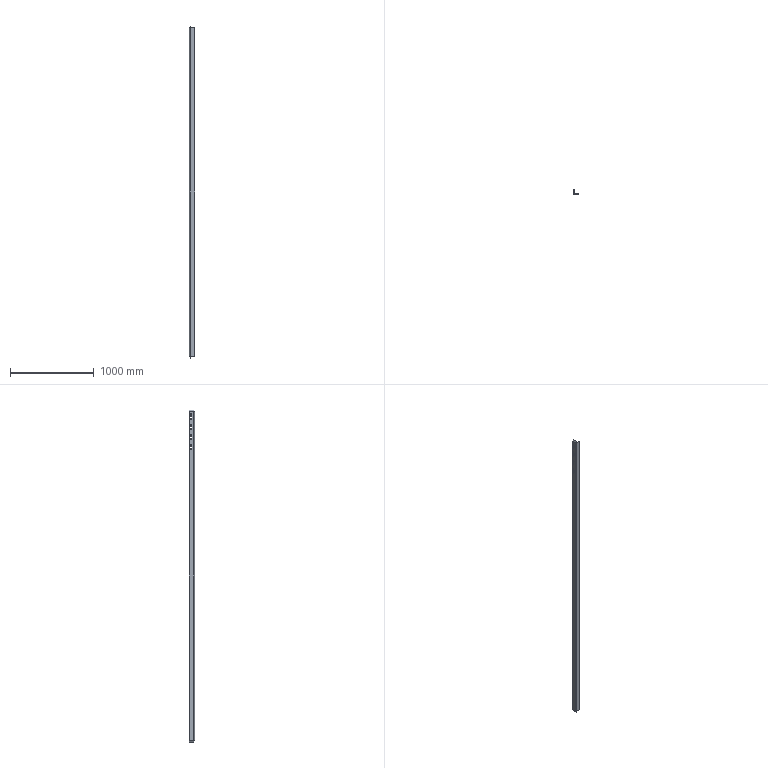Part | STEP file | BCC3 H12_1B | 1 solid | 96 faces | box 60 x 60 x 3968 mm | volume 2197436 mm3 | plane 42 | cylinder 38 | cone 16 | commonest cylinder face diameters 8 x19 6.5 x16 18 x3